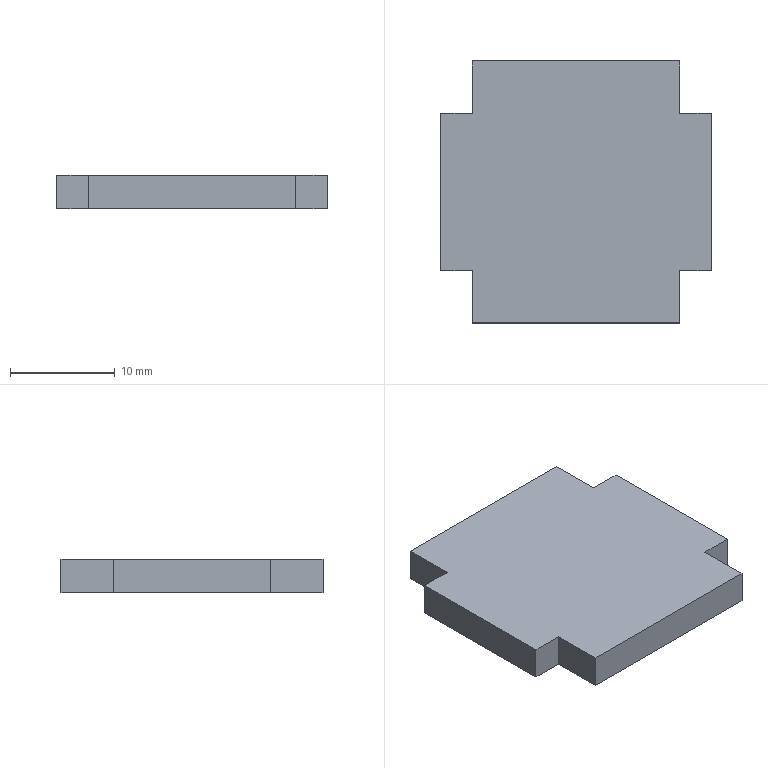Part | SolidWorks | features Extrusion 1 | 1 solid | 14 faces | box 25.8 x 25 x 3.2 mm | volume 1872 mm3 | plane 14
STEP:
#1=CARTESIAN_POINT('',(30.5,30.,-1.6));
#2=VERTEX_POINT('',#1);
#3=CARTESIAN_POINT('',(30.5,25.,-1.6));
#4=VERTEX_POINT('',#3);
#5=CARTESIAN_POINT('',(30.5,30.,-1.6));
#6=DIRECTION('',(0.,-1.,0.));
#7=VECTOR('',#6,1000.);
#8=LINE('',#5,#7);
#9=EDGE_CURVE('',#2,#4,#8,.T.);
#10=ORIENTED_EDGE('',*,*,#9,.T.);
#11=CARTESIAN_POINT('',(30.5,25.,1.6));
#12=VERTEX_POINT('',#11);
#13=CARTESIAN_POINT('',(30.5,25.,1.6));
#14=DIRECTION('',(0.,0.,-1.));
#15=VECTOR('',#14,1000.);
#16=LINE('',#13,#15);
#17=EDGE_CURVE('',#12,#4,#16,.T.);
#18=ORIENTED_EDGE('',*,*,#17,.F.);
#19=CARTESIAN_POINT('',(30.5,30.,1.6));
#20=VERTEX_POINT('',#19);
#21=CARTESIAN_POINT('',(30.5,30.,1.6));
#22=DIRECTION('',(0.,-1.,0.));
#23=VECTOR('',#22,1000.);
#24=LINE('',#21,#23);
#25=EDGE_CURVE('',#20,#12,#24,.T.);
#26=ORIENTED_EDGE('',*,*,#25,.F.);
#27=CARTESIAN_POINT('',(30.5,30.,1.6));
#28=DIRECTION('',(0.,0.,-1.));
#29=VECTOR('',#28,1000.);
#30=LINE('',#27,#29);
#31=EDGE_CURVE('',#20,#2,#30,.T.);
#32=ORIENTED_EDGE('',*,*,#31,.T.);
#33=EDGE_LOOP('',(#10,#18,#26,#32));
#34=FACE_OUTER_BOUND('',#33,.T.);
#35=CARTESIAN_POINT('',(30.5,30.,1.6));
#36=DIRECTION('',(1.,0.,0.));
#37=DIRECTION('',(0.,1.,0.));
#38=AXIS2_PLACEMENT_3D('',#35,#36,#37);
#39=PLANE('',#38);
#40=ADVANCED_FACE('',(#34),#39,.F.);
#41=CARTESIAN_POINT('',(50.3,25.,-1.6));
#42=VERTEX_POINT('',#41);
#43=CARTESIAN_POINT('',(30.5,25.,-1.6));
#44=DIRECTION('',(1.,0.,0.));
#45=VECTOR('',#44,1000.);
#46=LINE('',#43,#45);
#47=EDGE_CURVE('',#4,#42,#46,.T.);
#48=ORIENTED_EDGE('',*,*,#47,.T.);
#49=CARTESIAN_POINT('',(50.3,25.,1.6));
#50=VERTEX_POINT('',#49);
#51=CARTESIAN_POINT('',(50.3,25.,1.6));
#52=DIRECTION('',(0.,0.,-1.));
#53=VECTOR('',#52,1000.);
#54=LINE('',#51,#53);
#55=EDGE_CURVE('',#50,#42,#54,.T.);
#56=ORIENTED_EDGE('',*,*,#55,.F.);
#57=CARTESIAN_POINT('',(30.5,25.,1.6));
#58=DIRECTION('',(1.,0.,0.));
#59=VECTOR('',#58,1000.);
#60=LINE('',#57,#59);
#61=EDGE_CURVE('',#12,#50,#60,.T.);
#62=ORIENTED_EDGE('',*,*,#61,.F.);
#63=ORIENTED_EDGE('',*,*,#17,.T.);
#64=EDGE_LOOP('',(#48,#56,#62,#63));
#65=FACE_OUTER_BOUND('',#64,.T.);
#66=CARTESIAN_POINT('',(30.5,25.,1.6));
#67=DIRECTION('',(0.,1.,0.));
#68=DIRECTION('',(0.,0.,1.));
#69=AXIS2_PLACEMENT_3D('',#66,#67,#68);
#70=PLANE('',#69);
#71=ADVANCED_FACE('',(#65),#70,.F.);
#72=CARTESIAN_POINT('',(50.3,30.,-1.6));
#73=VERTEX_POINT('',#72);
#74=CARTESIAN_POINT('',(50.3,25.,-1.6));
#75=DIRECTION('',(0.,1.,0.));
#76=VECTOR('',#75,1000.);
#77=LINE('',#74,#76);
#78=EDGE_CURVE('',#42,#73,#77,.T.);
#79=ORIENTED_EDGE('',*,*,#78,.T.);
#80=CARTESIAN_POINT('',(50.3,30.,1.6));
#81=VERTEX_POINT('',#80);
#82=CARTESIAN_POINT('',(50.3,30.,1.6));
#83=DIRECTION('',(0.,0.,-1.));
#84=VECTOR('',#83,1000.);
#85=LINE('',#82,#84);
#86=EDGE_CURVE('',#81,#73,#85,.T.);
#87=ORIENTED_EDGE('',*,*,#86,.F.);
#88=CARTESIAN_POINT('',(50.3,25.,1.6));
#89=DIRECTION('',(0.,1.,0.));
#90=VECTOR('',#89,1000.);
#91=LINE('',#88,#90);
#92=EDGE_CURVE('',#50,#81,#91,.T.);
#93=ORIENTED_EDGE('',*,*,#92,.F.);
#94=ORIENTED_EDGE('',*,*,#55,.T.);
#95=EDGE_LOOP('',(#79,#87,#93,#94));
#96=FACE_OUTER_BOUND('',#95,.T.);
#97=CARTESIAN_POINT('',(50.3,25.,1.6));
#98=DIRECTION('',(-1.,0.,0.));
#99=DIRECTION('',(0.,0.,1.));
#100=AXIS2_PLACEMENT_3D('',#97,#98,#99);
#101=PLANE('',#100);
#102=ADVANCED_FACE('',(#96),#101,.F.);
#103=CARTESIAN_POINT('',(53.3,30.,-1.6));
#104=VERTEX_POINT('',#103);
#105=CARTESIAN_POINT('',(50.3,30.,-1.6));
#106=DIRECTION('',(1.,0.,0.));
#107=VECTOR('',#106,1000.);
#108=LINE('',#105,#107);
#109=EDGE_CURVE('',#73,#104,#108,.T.);
#110=ORIENTED_EDGE('',*,*,#109,.T.);
#111=CARTESIAN_POINT('',(53.3,30.,1.6));
#112=VERTEX_POINT('',#111);
#113=CARTESIAN_POINT('',(53.3,30.,1.6));
#114=DIRECTION('',(0.,0.,-1.));
#115=VECTOR('',#114,1000.);
#116=LINE('',#113,#115);
#117=EDGE_CURVE('',#112,#104,#116,.T.);
#118=ORIENTED_EDGE('',*,*,#117,.F.);
#119=CARTESIAN_POINT('',(50.3,30.,1.6));
#120=DIRECTION('',(1.,0.,0.));
#121=VECTOR('',#120,1000.);
#122=LINE('',#119,#121);
#123=EDGE_CURVE('',#81,#112,#122,.T.);
#124=ORIENTED_EDGE('',*,*,#123,.F.);
#125=ORIENTED_EDGE('',*,*,#86,.T.);
#126=EDGE_LOOP('',(#110,#118,#124,#125));
#127=FACE_OUTER_BOUND('',#126,.T.);
#128=CARTESIAN_POINT('',(50.3,30.,1.6));
#129=DIRECTION('',(0.,1.,0.));
#130=DIRECTION('',(0.,0.,1.));
#131=AXIS2_PLACEMENT_3D('',#128,#129,#130);
#132=PLANE('',#131);
#133=ADVANCED_FACE('',(#127),#132,.F.);
#134=CARTESIAN_POINT('',(53.3,45.,-1.6));
#135=VERTEX_POINT('',#134);
#136=CARTESIAN_POINT('',(53.3,30.,-1.6));
#137=DIRECTION('',(0.,1.,0.));
#138=VECTOR('',#137,1000.);
#139=LINE('',#136,#138);
#140=EDGE_CURVE('',#104,#135,#139,.T.);
#141=ORIENTED_EDGE('',*,*,#140,.T.);
#142=CARTESIAN_POINT('',(53.3,45.,1.6));
#143=VERTEX_POINT('',#142);
#144=CARTESIAN_POINT('',(53.3,45.,1.6));
#145=DIRECTION('',(0.,0.,-1.));
#146=VECTOR('',#145,1000.);
#147=LINE('',#144,#146);
#148=EDGE_CURVE('',#143,#135,#147,.T.);
#149=ORIENTED_EDGE('',*,*,#148,.F.);
#150=CARTESIAN_POINT('',(53.3,30.,1.6));
#151=DIRECTION('',(0.,1.,0.));
#152=VECTOR('',#151,1000.);
#153=LINE('',#150,#152);
#154=EDGE_CURVE('',#112,#143,#153,.T.);
#155=ORIENTED_EDGE('',*,*,#154,.F.);
#156=ORIENTED_EDGE('',*,*,#117,.T.);
#157=EDGE_LOOP('',(#141,#149,#155,#156));
#158=FACE_OUTER_BOUND('',#157,.T.);
#159=CARTESIAN_POINT('',(53.3,30.,1.6));
#160=DIRECTION('',(-1.,0.,0.));
#161=DIRECTION('',(0.,0.,1.));
#162=AXIS2_PLACEMENT_3D('',#159,#160,#161);
#163=PLANE('',#162);
#164=ADVANCED_FACE('',(#158),#163,.F.);
#165=CARTESIAN_POINT('',(50.3,45.,-1.6));
#166=VERTEX_POINT('',#165);
#167=CARTESIAN_POINT('',(53.3,45.,-1.6));
#168=DIRECTION('',(-1.,0.,0.));
#169=VECTOR('',#168,1000.);
#170=LINE('',#167,#169);
#171=EDGE_CURVE('',#135,#166,#170,.T.);
#172=ORIENTED_EDGE('',*,*,#171,.T.);
#173=CARTESIAN_POINT('',(50.3,45.,1.6));
#174=VERTEX_POINT('',#173);
#175=CARTESIAN_POINT('',(50.3,45.,1.6));
#176=DIRECTION('',(0.,0.,-1.));
#177=VECTOR('',#176,1000.);
#178=LINE('',#175,#177);
#179=EDGE_CURVE('',#174,#166,#178,.T.);
#180=ORIENTED_EDGE('',*,*,#179,.F.);
#181=CARTESIAN_POINT('',(53.3,45.,1.6));
#182=DIRECTION('',(-1.,0.,0.));
#183=VECTOR('',#182,1000.);
#184=LINE('',#181,#183);
#185=EDGE_CURVE('',#143,#174,#184,.T.);
#186=ORIENTED_EDGE('',*,*,#185,.F.);
#187=ORIENTED_EDGE('',*,*,#148,.T.);
#188=EDGE_LOOP('',(#172,#180,#186,#187));
#189=FACE_OUTER_BOUND('',#188,.T.);
#190=CARTESIAN_POINT('',(53.3,45.,1.6));
#191=DIRECTION('',(0.,-1.,0.));
#192=DIRECTION('',(0.,0.,-1.));
#193=AXIS2_PLACEMENT_3D('',#190,#191,#192);
#194=PLANE('',#193);
#195=ADVANCED_FACE('',(#189),#194,.F.);
#196=CARTESIAN_POINT('',(50.3,50.,-1.6));
#197=VERTEX_POINT('',#196);
#198=CARTESIAN_POINT('',(50.3,45.,-1.6));
#199=DIRECTION('',(0.,1.,0.));
#200=VECTOR('',#199,1000.);
#201=LINE('',#198,#200);
#202=EDGE_CURVE('',#166,#197,#201,.T.);
#203=ORIENTED_EDGE('',*,*,#202,.T.);
#204=CARTESIAN_POINT('',(50.3,50.,1.6));
#205=VERTEX_POINT('',#204);
#206=CARTESIAN_POINT('',(50.3,50.,1.6));
#207=DIRECTION('',(0.,0.,-1.));
#208=VECTOR('',#207,1000.);
#209=LINE('',#206,#208);
#210=EDGE_CURVE('',#205,#197,#209,.T.);
#211=ORIENTED_EDGE('',*,*,#210,.F.);
#212=CARTESIAN_POINT('',(50.3,45.,1.6));
#213=DIRECTION('',(0.,1.,0.));
#214=VECTOR('',#213,1000.);
#215=LINE('',#212,#214);
#216=EDGE_CURVE('',#174,#205,#215,.T.);
#217=ORIENTED_EDGE('',*,*,#216,.F.);
#218=ORIENTED_EDGE('',*,*,#179,.T.);
#219=EDGE_LOOP('',(#203,#211,#217,#218));
#220=FACE_OUTER_BOUND('',#219,.T.);
#221=CARTESIAN_POINT('',(50.3,45.,1.6));
#222=DIRECTION('',(-1.,0.,0.));
#223=DIRECTION('',(0.,-1.,0.));
#224=AXIS2_PLACEMENT_3D('',#221,#222,#223);
#225=PLANE('',#224);
#226=ADVANCED_FACE('',(#220),#225,.F.);
#227=CARTESIAN_POINT('',(30.5,50.,-1.6));
#228=VERTEX_POINT('',#227);
#229=CARTESIAN_POINT('',(50.3,50.,-1.6));
#230=DIRECTION('',(-1.,0.,0.));
#231=VECTOR('',#230,1000.);
#232=LINE('',#229,#231);
#233=EDGE_CURVE('',#197,#228,#232,.T.);
#234=ORIENTED_EDGE('',*,*,#233,.T.);
#235=CARTESIAN_POINT('',(30.5,50.,1.6));
#236=VERTEX_POINT('',#235);
#237=CARTESIAN_POINT('',(30.5,50.,1.6));
#238=DIRECTION('',(0.,0.,-1.));
#239=VECTOR('',#238,1000.);
#240=LINE('',#237,#239);
#241=EDGE_CURVE('',#236,#228,#240,.T.);
#242=ORIENTED_EDGE('',*,*,#241,.F.);
#243=CARTESIAN_POINT('',(50.3,50.,1.6));
#244=DIRECTION('',(-1.,0.,0.));
#245=VECTOR('',#244,1000.);
#246=LINE('',#243,#245);
#247=EDGE_CURVE('',#205,#236,#246,.T.);
#248=ORIENTED_EDGE('',*,*,#247,.F.);
#249=ORIENTED_EDGE('',*,*,#210,.T.);
#250=EDGE_LOOP('',(#234,#242,#248,#249));
#251=FACE_OUTER_BOUND('',#250,.T.);
#252=CARTESIAN_POINT('',(50.3,50.,1.6));
#253=DIRECTION('',(0.,-1.,0.));
#254=DIRECTION('',(0.,0.,-1.));
#255=AXIS2_PLACEMENT_3D('',#252,#253,#254);
#256=PLANE('',#255);
#257=ADVANCED_FACE('',(#251),#256,.F.);
#258=CARTESIAN_POINT('',(30.5,45.,-1.6));
#259=VERTEX_POINT('',#258);
#260=CARTESIAN_POINT('',(30.5,50.,-1.6));
#261=DIRECTION('',(0.,-1.,0.));
#262=VECTOR('',#261,1000.);
#263=LINE('',#260,#262);
#264=EDGE_CURVE('',#228,#259,#263,.T.);
#265=ORIENTED_EDGE('',*,*,#264,.T.);
#266=CARTESIAN_POINT('',(30.5,45.,1.6));
#267=VERTEX_POINT('',#266);
#268=CARTESIAN_POINT('',(30.5,45.,1.6));
#269=DIRECTION('',(0.,0.,-1.));
#270=VECTOR('',#269,1000.);
#271=LINE('',#268,#270);
#272=EDGE_CURVE('',#267,#259,#271,.T.);
#273=ORIENTED_EDGE('',*,*,#272,.F.);
#274=CARTESIAN_POINT('',(30.5,50.,1.6));
#275=DIRECTION('',(0.,-1.,0.));
#276=VECTOR('',#275,1000.);
#277=LINE('',#274,#276);
#278=EDGE_CURVE('',#236,#267,#277,.T.);
#279=ORIENTED_EDGE('',*,*,#278,.F.);
#280=ORIENTED_EDGE('',*,*,#241,.T.);
#281=EDGE_LOOP('',(#265,#273,#279,#280));
#282=FACE_OUTER_BOUND('',#281,.T.);
#283=CARTESIAN_POINT('',(30.5,50.,1.6));
#284=DIRECTION('',(1.,0.,0.));
#285=DIRECTION('',(0.,0.,-1.));
#286=AXIS2_PLACEMENT_3D('',#283,#284,#285);
#287=PLANE('',#286);
#288=ADVANCED_FACE('',(#282),#287,.F.);
#289=CARTESIAN_POINT('',(27.5,45.,-1.6));
#290=VERTEX_POINT('',#289);
#291=CARTESIAN_POINT('',(27.5,45.,-1.6));
#292=DIRECTION('',(-1.,0.,0.));
#293=VECTOR('',#292,1000.);
#294=LINE('',#291,#293);
#295=EDGE_CURVE('',#259,#290,#294,.T.);
#296=ORIENTED_EDGE('',*,*,#295,.T.);
#297=CARTESIAN_POINT('',(27.5,45.,1.6));
#298=VERTEX_POINT('',#297);
#299=CARTESIAN_POINT('',(27.5,45.,1.6));
#300=DIRECTION('',(0.,0.,-1.));
#301=VECTOR('',#300,1000.);
#302=LINE('',#299,#301);
#303=EDGE_CURVE('',#298,#290,#302,.T.);
#304=ORIENTED_EDGE('',*,*,#303,.F.);
#305=CARTESIAN_POINT('',(27.5,45.,1.6));
#306=DIRECTION('',(-1.,0.,0.));
#307=VECTOR('',#306,1000.);
#308=LINE('',#305,#307);
#309=EDGE_CURVE('',#267,#298,#308,.T.);
#310=ORIENTED_EDGE('',*,*,#309,.F.);
#311=ORIENTED_EDGE('',*,*,#272,.T.);
#312=EDGE_LOOP('',(#296,#304,#310,#311));
#313=FACE_OUTER_BOUND('',#312,.T.);
#314=CARTESIAN_POINT('',(27.5,45.,1.6));
#315=DIRECTION('',(0.,-1.,0.));
#316=DIRECTION('',(0.,0.,-1.));
#317=AXIS2_PLACEMENT_3D('',#314,#315,#316);
#318=PLANE('',#317);
#319=ADVANCED_FACE('',(#313),#318,.F.);
#320=CARTESIAN_POINT('',(27.5,30.,-1.6));
#321=VERTEX_POINT('',#320);
#322=CARTESIAN_POINT('',(27.5,30.,-1.6));
#323=DIRECTION('',(0.,-1.,0.));
#324=VECTOR('',#323,1000.);
#325=LINE('',#322,#324);
#326=EDGE_CURVE('',#290,#321,#325,.T.);
#327=ORIENTED_EDGE('',*,*,#326,.T.);
#328=CARTESIAN_POINT('',(27.5,30.,1.6));
#329=VERTEX_POINT('',#328);
#330=CARTESIAN_POINT('',(27.5,30.,1.6));
#331=DIRECTION('',(0.,0.,-1.));
#332=VECTOR('',#331,1000.);
#333=LINE('',#330,#332);
#334=EDGE_CURVE('',#329,#321,#333,.T.);
#335=ORIENTED_EDGE('',*,*,#334,.F.);
#336=CARTESIAN_POINT('',(27.5,30.,1.6));
#337=DIRECTION('',(0.,-1.,0.));
#338=VECTOR('',#337,1000.);
#339=LINE('',#336,#338);
#340=EDGE_CURVE('',#298,#329,#339,.T.);
#341=ORIENTED_EDGE('',*,*,#340,.F.);
#342=ORIENTED_EDGE('',*,*,#303,.T.);
#343=EDGE_LOOP('',(#327,#335,#341,#342));
#344=FACE_OUTER_BOUND('',#343,.T.);
#345=CARTESIAN_POINT('',(27.5,30.,1.6));
#346=DIRECTION('',(1.,0.,0.));
#347=DIRECTION('',(0.,0.,-1.));
#348=AXIS2_PLACEMENT_3D('',#345,#346,#347);
#349=PLANE('',#348);
#350=ADVANCED_FACE('',(#344),#349,.F.);
#351=CARTESIAN_POINT('',(30.5,30.,-1.6));
#352=DIRECTION('',(1.,0.,0.));
#353=VECTOR('',#352,1000.);
#354=LINE('',#351,#353);
#355=EDGE_CURVE('',#321,#2,#354,.T.);
#356=ORIENTED_EDGE('',*,*,#355,.T.);
#357=ORIENTED_EDGE('',*,*,#31,.F.);
#358=CARTESIAN_POINT('',(30.5,30.,1.6));
#359=DIRECTION('',(1.,0.,0.));
#360=VECTOR('',#359,1000.);
#361=LINE('',#358,#360);
#362=EDGE_CURVE('',#329,#20,#361,.T.);
#363=ORIENTED_EDGE('',*,*,#362,.F.);
#364=ORIENTED_EDGE('',*,*,#334,.T.);
#365=EDGE_LOOP('',(#356,#357,#363,#364));
#366=FACE_OUTER_BOUND('',#365,.T.);
#367=CARTESIAN_POINT('',(30.5,30.,1.6));
#368=DIRECTION('',(0.,1.,0.));
#369=DIRECTION('',(0.,0.,1.));
#370=AXIS2_PLACEMENT_3D('',#367,#368,#369);
#371=PLANE('',#370);
#372=ADVANCED_FACE('',(#366),#371,.F.);
#373=ORIENTED_EDGE('',*,*,#25,.T.);
#374=ORIENTED_EDGE('',*,*,#61,.T.);
#375=ORIENTED_EDGE('',*,*,#92,.T.);
#376=ORIENTED_EDGE('',*,*,#123,.T.);
#377=ORIENTED_EDGE('',*,*,#154,.T.);
#378=ORIENTED_EDGE('',*,*,#185,.T.);
#379=ORIENTED_EDGE('',*,*,#216,.T.);
#380=ORIENTED_EDGE('',*,*,#247,.T.);
#381=ORIENTED_EDGE('',*,*,#278,.T.);
#382=ORIENTED_EDGE('',*,*,#309,.T.);
#383=ORIENTED_EDGE('',*,*,#340,.T.);
#384=ORIENTED_EDGE('',*,*,#362,.T.);
#385=EDGE_LOOP('',(#373,#374,#375,#376,#377,#378,#379,#380,#381,#382,#383,#384));
#386=FACE_OUTER_BOUND('',#385,.T.);
#387=CARTESIAN_POINT('',(0.,0.,1.6));
#388=DIRECTION('',(0.,0.,1.));
#389=DIRECTION('',(1.,0.,0.));
#390=AXIS2_PLACEMENT_3D('',#387,#388,#389);
#391=PLANE('',#390);
#392=ADVANCED_FACE('',(#386),#391,.T.);
#393=ORIENTED_EDGE('',*,*,#9,.F.);
#394=ORIENTED_EDGE('',*,*,#355,.F.);
#395=ORIENTED_EDGE('',*,*,#326,.F.);
#396=ORIENTED_EDGE('',*,*,#295,.F.);
#397=ORIENTED_EDGE('',*,*,#264,.F.);
#398=ORIENTED_EDGE('',*,*,#233,.F.);
#399=ORIENTED_EDGE('',*,*,#202,.F.);
#400=ORIENTED_EDGE('',*,*,#171,.F.);
#401=ORIENTED_EDGE('',*,*,#140,.F.);
#402=ORIENTED_EDGE('',*,*,#109,.F.);
#403=ORIENTED_EDGE('',*,*,#78,.F.);
#404=ORIENTED_EDGE('',*,*,#47,.F.);
#405=EDGE_LOOP('',(#393,#394,#395,#396,#397,#398,#399,#400,#401,#402,#403,#404));
#406=FACE_OUTER_BOUND('',#405,.T.);
#407=CARTESIAN_POINT('',(0.,0.,-1.6));
#408=DIRECTION('',(0.,0.,1.));
#409=DIRECTION('',(1.,0.,0.));
#410=AXIS2_PLACEMENT_3D('',#407,#408,#409);
#411=PLANE('',#410);
#412=ADVANCED_FACE('',(#406),#411,.F.);
#413=CLOSED_SHELL('',(#40,#71,#102,#133,#164,#195,#226,#257,#288,#319,#350,#372,#392,#412));
#414=MANIFOLD_SOLID_BREP('',#413);
#415=CARTESIAN_POINT('',(0.,0.,0.));
#416=DIRECTION('',(0.,0.,1.));
#417=DIRECTION('',(1.,0.,0.));
#418=AXIS2_PLACEMENT_3D('',#415,#416,#417);
#419=(LENGTH_UNIT()NAMED_UNIT(*)SI_UNIT(.MILLI.,.METRE.));
#420=UNCERTAINTY_MEASURE_WITH_UNIT(LENGTH_MEASURE(0.00001),#419,'','');
#421=(NAMED_UNIT(*)PLANE_ANGLE_UNIT()SI_UNIT($,.RADIAN.));
#422=(NAMED_UNIT(*)SI_UNIT($,.STERADIAN.)SOLID_ANGLE_UNIT());
#423=(GEOMETRIC_REPRESENTATION_CONTEXT(3)GLOBAL_UNCERTAINTY_ASSIGNED_CONTEXT((#420))GLOBAL_UNIT_ASSIGNED_CONTEXT((#419,#421,#422))REPRESENTATION_CONTEXT('',''));
#424=ADVANCED_BREP_SHAPE_REPRESENTATION('',(#414,#418),#423);